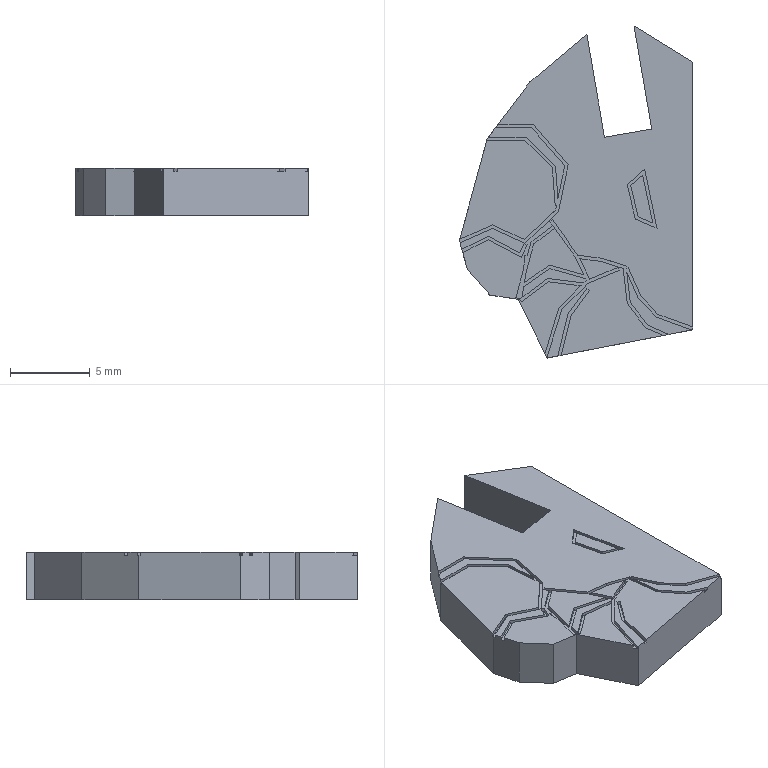Part | SolidWorks | features BaseBody 1 | 1 solid | 134 faces | box 14.575 x 20.753 x 3 mm | volume 629.873 mm3 | plane 134